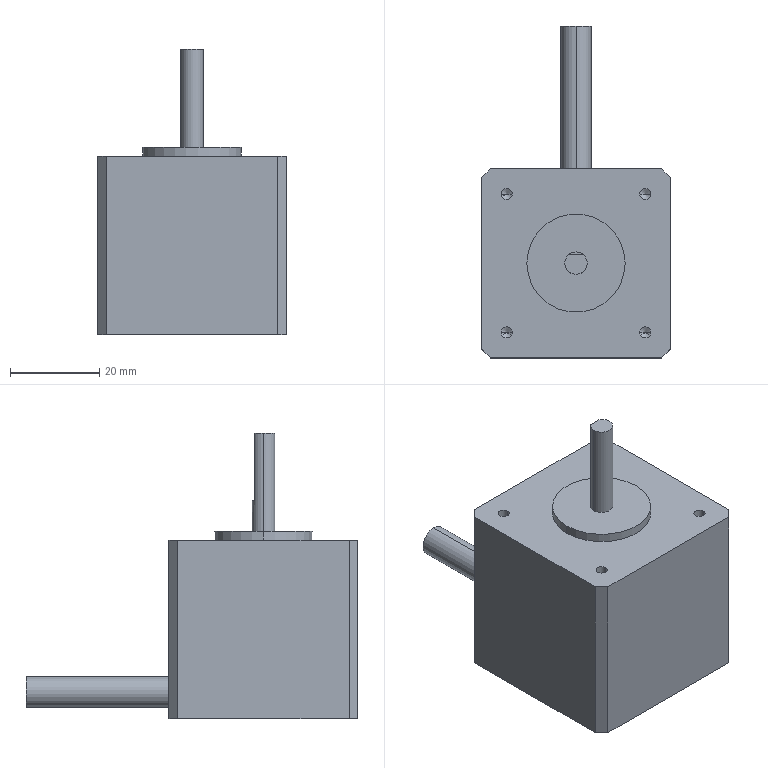Part | NX | features BREP 1 | 1 solid | 37 faces | box 42.3 x 74.3 x 64 mm | volume 73352 mm3 | plane 15 | cylinder 14 | cone 8 | commonest cylinder face diameters 2.5 x8 5 x2 6.776 x2 22 x2
STEP:
#1=CARTESIAN_POINT('',(0.,53.15,2.645));
#2=VERTEX_POINT('',#1);
#3=CARTESIAN_POINT('',(0.,53.15,9.422));
#4=VERTEX_POINT('',#3);
#5=CARTESIAN_POINT('',(0.,53.15,6.033));
#6=DIRECTION('',(0.,1.,0.));
#7=DIRECTION('',(0.,0.,1.));
#8=AXIS2_PLACEMENT_3D('',#5,#6,#7);
#9=CIRCLE('',#8,3.388);
#10=EDGE_CURVE('',#2,#4,#9,.T.);
#11=ORIENTED_EDGE('',*,*,#10,.T.);
#12=CARTESIAN_POINT('',(0.,53.15,6.033));
#13=DIRECTION('',(0.,1.,0.));
#14=DIRECTION('',(0.,0.,1.));
#15=AXIS2_PLACEMENT_3D('',#12,#13,#14);
#16=CIRCLE('',#15,3.388);
#17=EDGE_CURVE('',#4,#2,#16,.T.);
#18=ORIENTED_EDGE('',*,*,#17,.T.);
#19=EDGE_LOOP('',(#11,#18));
#20=FACE_BOUND('',#19,.T.);
#21=CARTESIAN_POINT('',(0.,53.15,6.033));
#22=DIRECTION('',(0.,1.,0.));
#23=DIRECTION('',(0.,0.,1.));
#24=AXIS2_PLACEMENT_3D('',#21,#22,#23);
#25=PLANE('',#24);
#26=ADVANCED_FACE('',(#20),#25,.T.);
#27=CARTESIAN_POINT('',(0.,21.15,9.422));
#28=VERTEX_POINT('',#27);
#29=CARTESIAN_POINT('',(0.,53.15,9.422));
#30=DIRECTION('',(0.,-1.,0.));
#31=VECTOR('',#30,1000.);
#32=LINE('',#29,#31);
#33=EDGE_CURVE('',#4,#28,#32,.T.);
#34=ORIENTED_EDGE('',*,*,#33,.F.);
#35=ORIENTED_EDGE('',*,*,#10,.F.);
#36=CARTESIAN_POINT('',(0.,21.15,2.645));
#37=VERTEX_POINT('',#36);
#38=CARTESIAN_POINT('',(0.,53.15,2.645));
#39=DIRECTION('',(0.,-1.,0.));
#40=VECTOR('',#39,1000.);
#41=LINE('',#38,#40);
#42=EDGE_CURVE('',#2,#37,#41,.T.);
#43=ORIENTED_EDGE('',*,*,#42,.T.);
#44=CARTESIAN_POINT('',(0.,21.15,6.033));
#45=DIRECTION('',(0.,1.,0.));
#46=DIRECTION('',(0.,0.,-1.));
#47=AXIS2_PLACEMENT_3D('',#44,#45,#46);
#48=CIRCLE('',#47,3.388);
#49=EDGE_CURVE('',#37,#28,#48,.T.);
#50=ORIENTED_EDGE('',*,*,#49,.T.);
#51=EDGE_LOOP('',(#34,#35,#43,#50));
#52=FACE_BOUND('',#51,.T.);
#53=CARTESIAN_POINT('',(0.,53.15,6.033));
#54=DIRECTION('',(0.,-1.,0.));
#55=DIRECTION('',(0.,0.,-1.));
#56=AXIS2_PLACEMENT_3D('',#53,#54,#55);
#57=CYLINDRICAL_SURFACE('',#56,3.388);
#58=ADVANCED_FACE('',(#52),#57,.T.);
#59=CARTESIAN_POINT('',(-19.15,21.15,40.));
#60=VERTEX_POINT('',#59);
#61=CARTESIAN_POINT('',(-21.15,19.15,40.));
#62=VERTEX_POINT('',#61);
#63=CARTESIAN_POINT('',(-21.15,19.15,40.));
#64=DIRECTION('',(-0.7071,-0.7071,0.));
#65=VECTOR('',#64,1000.);
#66=LINE('',#63,#65);
#67=EDGE_CURVE('',#60,#62,#66,.T.);
#68=ORIENTED_EDGE('',*,*,#67,.F.);
#69=CARTESIAN_POINT('',(-19.15,21.15,0.));
#70=VERTEX_POINT('',#69);
#71=CARTESIAN_POINT('',(-19.15,21.15,40.));
#72=DIRECTION('',(0.,0.,1.));
#73=VECTOR('',#72,1000.);
#74=LINE('',#71,#73);
#75=EDGE_CURVE('',#70,#60,#74,.T.);
#76=ORIENTED_EDGE('',*,*,#75,.F.);
#77=CARTESIAN_POINT('',(-21.15,19.15,0.));
#78=VERTEX_POINT('',#77);
#79=CARTESIAN_POINT('',(-20.15,20.15,0.));
#80=DIRECTION('',(0.7071,0.7071,0.));
#81=VECTOR('',#80,1000.);
#82=LINE('',#79,#81);
#83=EDGE_CURVE('',#78,#70,#82,.T.);
#84=ORIENTED_EDGE('',*,*,#83,.F.);
#85=CARTESIAN_POINT('',(-21.15,19.15,40.));
#86=DIRECTION('',(0.,0.,-1.));
#87=VECTOR('',#86,1000.);
#88=LINE('',#85,#87);
#89=EDGE_CURVE('',#62,#78,#88,.T.);
#90=ORIENTED_EDGE('',*,*,#89,.F.);
#91=EDGE_LOOP('',(#68,#76,#84,#90));
#92=FACE_BOUND('',#91,.T.);
#93=CARTESIAN_POINT('',(-21.15,19.15,40.));
#94=DIRECTION('',(0.7071,-0.7071,0.));
#95=DIRECTION('',(0.,0.,-1.));
#96=AXIS2_PLACEMENT_3D('',#93,#94,#95);
#97=PLANE('',#96);
#98=ADVANCED_FACE('',(#92),#97,.F.);
#99=CARTESIAN_POINT('',(21.15,19.15,40.));
#100=VERTEX_POINT('',#99);
#101=CARTESIAN_POINT('',(19.15,21.15,40.));
#102=VERTEX_POINT('',#101);
#103=CARTESIAN_POINT('',(19.15,21.15,40.));
#104=DIRECTION('',(-0.7071,0.7071,0.));
#105=VECTOR('',#104,1000.);
#106=LINE('',#103,#105);
#107=EDGE_CURVE('',#100,#102,#106,.T.);
#108=ORIENTED_EDGE('',*,*,#107,.F.);
#109=CARTESIAN_POINT('',(21.15,19.15,0.));
#110=VERTEX_POINT('',#109);
#111=CARTESIAN_POINT('',(21.15,19.15,40.));
#112=DIRECTION('',(0.,0.,1.));
#113=VECTOR('',#112,1000.);
#114=LINE('',#111,#113);
#115=EDGE_CURVE('',#110,#100,#114,.T.);
#116=ORIENTED_EDGE('',*,*,#115,.F.);
#117=CARTESIAN_POINT('',(19.15,21.15,0.));
#118=VERTEX_POINT('',#117);
#119=CARTESIAN_POINT('',(20.15,20.15,0.));
#120=DIRECTION('',(0.7071,-0.7071,0.));
#121=VECTOR('',#120,1000.);
#122=LINE('',#119,#121);
#123=EDGE_CURVE('',#118,#110,#122,.T.);
#124=ORIENTED_EDGE('',*,*,#123,.F.);
#125=CARTESIAN_POINT('',(19.15,21.15,40.));
#126=DIRECTION('',(0.,0.,-1.));
#127=VECTOR('',#126,1000.);
#128=LINE('',#125,#127);
#129=EDGE_CURVE('',#102,#118,#128,.T.);
#130=ORIENTED_EDGE('',*,*,#129,.F.);
#131=EDGE_LOOP('',(#108,#116,#124,#130));
#132=FACE_BOUND('',#131,.T.);
#133=CARTESIAN_POINT('',(19.15,21.15,40.));
#134=DIRECTION('',(-0.7071,-0.7071,0.));
#135=DIRECTION('',(0.,0.,-1.));
#136=AXIS2_PLACEMENT_3D('',#133,#134,#135);
#137=PLANE('',#136);
#138=ADVANCED_FACE('',(#132),#137,.F.);
#139=CARTESIAN_POINT('',(-21.15,-19.15,40.));
#140=VERTEX_POINT('',#139);
#141=CARTESIAN_POINT('',(-19.15,-21.15,40.));
#142=VERTEX_POINT('',#141);
#143=CARTESIAN_POINT('',(-19.15,-21.15,40.));
#144=DIRECTION('',(0.7071,-0.7071,0.));
#145=VECTOR('',#144,1000.);
#146=LINE('',#143,#145);
#147=EDGE_CURVE('',#140,#142,#146,.T.);
#148=ORIENTED_EDGE('',*,*,#147,.F.);
#149=CARTESIAN_POINT('',(-21.15,-19.15,0.));
#150=VERTEX_POINT('',#149);
#151=CARTESIAN_POINT('',(-21.15,-19.15,40.));
#152=DIRECTION('',(0.,0.,1.));
#153=VECTOR('',#152,1000.);
#154=LINE('',#151,#153);
#155=EDGE_CURVE('',#150,#140,#154,.T.);
#156=ORIENTED_EDGE('',*,*,#155,.F.);
#157=CARTESIAN_POINT('',(-19.15,-21.15,0.));
#158=VERTEX_POINT('',#157);
#159=CARTESIAN_POINT('',(-20.15,-20.15,0.));
#160=DIRECTION('',(-0.7071,0.7071,0.));
#161=VECTOR('',#160,1000.);
#162=LINE('',#159,#161);
#163=EDGE_CURVE('',#158,#150,#162,.T.);
#164=ORIENTED_EDGE('',*,*,#163,.F.);
#165=CARTESIAN_POINT('',(-19.15,-21.15,40.));
#166=DIRECTION('',(0.,0.,-1.));
#167=VECTOR('',#166,1000.);
#168=LINE('',#165,#167);
#169=EDGE_CURVE('',#142,#158,#168,.T.);
#170=ORIENTED_EDGE('',*,*,#169,.F.);
#171=EDGE_LOOP('',(#148,#156,#164,#170));
#172=FACE_BOUND('',#171,.T.);
#173=CARTESIAN_POINT('',(-19.15,-21.15,40.));
#174=DIRECTION('',(0.7071,0.7071,0.));
#175=DIRECTION('',(0.,0.,-1.));
#176=AXIS2_PLACEMENT_3D('',#173,#174,#175);
#177=PLANE('',#176);
#178=ADVANCED_FACE('',(#172),#177,.F.);
#179=CARTESIAN_POINT('',(19.15,-21.15,40.));
#180=VERTEX_POINT('',#179);
#181=CARTESIAN_POINT('',(21.15,-19.15,40.));
#182=VERTEX_POINT('',#181);
#183=CARTESIAN_POINT('',(21.15,-19.15,40.));
#184=DIRECTION('',(0.7071,0.7071,0.));
#185=VECTOR('',#184,1000.);
#186=LINE('',#183,#185);
#187=EDGE_CURVE('',#180,#182,#186,.T.);
#188=ORIENTED_EDGE('',*,*,#187,.F.);
#189=CARTESIAN_POINT('',(19.15,-21.15,0.));
#190=VERTEX_POINT('',#189);
#191=CARTESIAN_POINT('',(19.15,-21.15,40.));
#192=DIRECTION('',(0.,0.,1.));
#193=VECTOR('',#192,1000.);
#194=LINE('',#191,#193);
#195=EDGE_CURVE('',#190,#180,#194,.T.);
#196=ORIENTED_EDGE('',*,*,#195,.F.);
#197=CARTESIAN_POINT('',(21.15,-19.15,0.));
#198=VERTEX_POINT('',#197);
#199=CARTESIAN_POINT('',(20.15,-20.15,0.));
#200=DIRECTION('',(-0.7071,-0.7071,0.));
#201=VECTOR('',#200,1000.);
#202=LINE('',#199,#201);
#203=EDGE_CURVE('',#198,#190,#202,.T.);
#204=ORIENTED_EDGE('',*,*,#203,.F.);
#205=CARTESIAN_POINT('',(21.15,-19.15,40.));
#206=DIRECTION('',(0.,0.,-1.));
#207=VECTOR('',#206,1000.);
#208=LINE('',#205,#207);
#209=EDGE_CURVE('',#182,#198,#208,.T.);
#210=ORIENTED_EDGE('',*,*,#209,.F.);
#211=EDGE_LOOP('',(#188,#196,#204,#210));
#212=FACE_BOUND('',#211,.T.);
#213=CARTESIAN_POINT('',(21.15,-19.15,40.));
#214=DIRECTION('',(-0.7071,0.7071,0.));
#215=DIRECTION('',(0.,0.,-1.));
#216=AXIS2_PLACEMENT_3D('',#213,#214,#215);
#217=PLANE('',#216);
#218=ADVANCED_FACE('',(#212),#217,.F.);
#219=CARTESIAN_POINT('',(-16.75,15.5,40.));
#220=VERTEX_POINT('',#219);
#221=CARTESIAN_POINT('',(-16.75,15.5,28.5));
#222=VERTEX_POINT('',#221);
#223=CARTESIAN_POINT('',(-16.75,15.5,40.));
#224=DIRECTION('',(0.,0.,1.));
#225=VECTOR('',#224,1000.);
#226=LINE('',#223,#225);
#227=EDGE_CURVE('',#220,#222,#226,.F.);
#228=ORIENTED_EDGE('',*,*,#227,.T.);
#229=CARTESIAN_POINT('',(-14.25,15.5,28.5));
#230=VERTEX_POINT('',#229);
#231=CARTESIAN_POINT('',(-15.5,15.5,28.5));
#232=DIRECTION('',(0.,0.,1.));
#233=DIRECTION('',(1.,0.,0.));
#234=AXIS2_PLACEMENT_3D('',#231,#232,#233);
#235=CIRCLE('',#234,1.25);
#236=EDGE_CURVE('',#230,#222,#235,.T.);
#237=ORIENTED_EDGE('',*,*,#236,.F.);
#238=CARTESIAN_POINT('',(-14.25,15.5,40.));
#239=VERTEX_POINT('',#238);
#240=CARTESIAN_POINT('',(-14.25,15.5,40.));
#241=DIRECTION('',(0.,0.,1.));
#242=VECTOR('',#241,1000.);
#243=LINE('',#240,#242);
#244=EDGE_CURVE('',#239,#230,#243,.F.);
#245=ORIENTED_EDGE('',*,*,#244,.F.);
#246=CARTESIAN_POINT('',(-15.5,15.5,40.));
#247=DIRECTION('',(0.,0.,1.));
#248=DIRECTION('',(1.,0.,0.));
#249=AXIS2_PLACEMENT_3D('',#246,#247,#248);
#250=CIRCLE('',#249,1.25);
#251=EDGE_CURVE('',#239,#220,#250,.T.);
#252=ORIENTED_EDGE('',*,*,#251,.T.);
#253=EDGE_LOOP('',(#228,#237,#245,#252));
#254=FACE_BOUND('',#253,.T.);
#255=CARTESIAN_POINT('',(-15.5,15.5,40.));
#256=DIRECTION('',(0.,0.,1.));
#257=DIRECTION('',(1.,0.,0.));
#258=AXIS2_PLACEMENT_3D('',#255,#256,#257);
#259=CYLINDRICAL_SURFACE('',#258,1.25);
#260=ADVANCED_FACE('',(#254),#259,.F.);
#261=CARTESIAN_POINT('',(-15.5,15.5,27.749));
#262=VERTEX_POINT('',#261);
#263=CARTESIAN_POINT('',(-16.75,15.5,28.5));
#264=DIRECTION('',(-0.8572,0.,0.515));
#265=VECTOR('',#264,1000.);
#266=LINE('',#263,#265);
#267=EDGE_CURVE('',#262,#222,#266,.T.);
#268=ORIENTED_EDGE('',*,*,#267,.F.);
#269=CARTESIAN_POINT('',(-14.25,15.5,28.5));
#270=DIRECTION('',(0.8572,0.,0.515));
#271=VECTOR('',#270,1000.);
#272=LINE('',#269,#271);
#273=EDGE_CURVE('',#262,#230,#272,.T.);
#274=ORIENTED_EDGE('',*,*,#273,.T.);
#275=ORIENTED_EDGE('',*,*,#236,.T.);
#276=EDGE_LOOP('',(#268,#274,#275));
#277=FACE_BOUND('',#276,.T.);
#278=CARTESIAN_POINT('',(-15.5,15.5,28.5));
#279=DIRECTION('',(0.,0.,1.));
#280=DIRECTION('',(1.,0.,0.));
#281=AXIS2_PLACEMENT_3D('',#278,#279,#280);
#282=CONICAL_SURFACE('',#281,1.25,1.03);
#283=ADVANCED_FACE('',(#277),#282,.F.);
#284=CARTESIAN_POINT('',(14.25,15.5,40.));
#285=VERTEX_POINT('',#284);
#286=CARTESIAN_POINT('',(14.25,15.5,28.5));
#287=VERTEX_POINT('',#286);
#288=CARTESIAN_POINT('',(14.25,15.5,40.));
#289=DIRECTION('',(0.,0.,1.));
#290=VECTOR('',#289,1000.);
#291=LINE('',#288,#290);
#292=EDGE_CURVE('',#285,#287,#291,.F.);
#293=ORIENTED_EDGE('',*,*,#292,.T.);
#294=CARTESIAN_POINT('',(16.75,15.5,28.5));
#295=VERTEX_POINT('',#294);
#296=CARTESIAN_POINT('',(15.5,15.5,28.5));
#297=DIRECTION('',(0.,0.,1.));
#298=DIRECTION('',(1.,0.,0.));
#299=AXIS2_PLACEMENT_3D('',#296,#297,#298);
#300=CIRCLE('',#299,1.25);
#301=EDGE_CURVE('',#295,#287,#300,.T.);
#302=ORIENTED_EDGE('',*,*,#301,.F.);
#303=CARTESIAN_POINT('',(16.75,15.5,40.));
#304=VERTEX_POINT('',#303);
#305=CARTESIAN_POINT('',(16.75,15.5,40.));
#306=DIRECTION('',(0.,0.,1.));
#307=VECTOR('',#306,1000.);
#308=LINE('',#305,#307);
#309=EDGE_CURVE('',#304,#295,#308,.F.);
#310=ORIENTED_EDGE('',*,*,#309,.F.);
#311=CARTESIAN_POINT('',(15.5,15.5,40.));
#312=DIRECTION('',(0.,0.,1.));
#313=DIRECTION('',(1.,0.,0.));
#314=AXIS2_PLACEMENT_3D('',#311,#312,#313);
#315=CIRCLE('',#314,1.25);
#316=EDGE_CURVE('',#304,#285,#315,.T.);
#317=ORIENTED_EDGE('',*,*,#316,.T.);
#318=EDGE_LOOP('',(#293,#302,#310,#317));
#319=FACE_BOUND('',#318,.T.);
#320=CARTESIAN_POINT('',(15.5,15.5,40.));
#321=DIRECTION('',(0.,0.,1.));
#322=DIRECTION('',(1.,0.,0.));
#323=AXIS2_PLACEMENT_3D('',#320,#321,#322);
#324=CYLINDRICAL_SURFACE('',#323,1.25);
#325=ADVANCED_FACE('',(#319),#324,.F.);
#326=CARTESIAN_POINT('',(15.5,15.5,27.749));
#327=VERTEX_POINT('',#326);
#328=CARTESIAN_POINT('',(14.25,15.5,28.5));
#329=DIRECTION('',(-0.8572,0.,0.515));
#330=VECTOR('',#329,1000.);
#331=LINE('',#328,#330);
#332=EDGE_CURVE('',#327,#287,#331,.T.);
#333=ORIENTED_EDGE('',*,*,#332,.F.);
#334=CARTESIAN_POINT('',(16.75,15.5,28.5));
#335=DIRECTION('',(0.8572,0.,0.515));
#336=VECTOR('',#335,1000.);
#337=LINE('',#334,#336);
#338=EDGE_CURVE('',#327,#295,#337,.T.);
#339=ORIENTED_EDGE('',*,*,#338,.T.);
#340=ORIENTED_EDGE('',*,*,#301,.T.);
#341=EDGE_LOOP('',(#333,#339,#340));
#342=FACE_BOUND('',#341,.T.);
#343=CARTESIAN_POINT('',(15.5,15.5,28.5));
#344=DIRECTION('',(0.,0.,1.));
#345=DIRECTION('',(1.,0.,0.));
#346=AXIS2_PLACEMENT_3D('',#343,#344,#345);
#347=CONICAL_SURFACE('',#346,1.25,1.03);
#348=ADVANCED_FACE('',(#342),#347,.F.);
#349=CARTESIAN_POINT('',(14.25,-15.5,40.));
#350=VERTEX_POINT('',#349);
#351=CARTESIAN_POINT('',(14.25,-15.5,28.5));
#352=VERTEX_POINT('',#351);
#353=CARTESIAN_POINT('',(14.25,-15.5,40.));
#354=DIRECTION('',(0.,0.,1.));
#355=VECTOR('',#354,1000.);
#356=LINE('',#353,#355);
#357=EDGE_CURVE('',#350,#352,#356,.F.);
#358=ORIENTED_EDGE('',*,*,#357,.T.);
#359=CARTESIAN_POINT('',(16.75,-15.5,28.5));
#360=VERTEX_POINT('',#359);
#361=CARTESIAN_POINT('',(15.5,-15.5,28.5));
#362=DIRECTION('',(0.,0.,1.));
#363=DIRECTION('',(1.,0.,0.));
#364=AXIS2_PLACEMENT_3D('',#361,#362,#363);
#365=CIRCLE('',#364,1.25);
#366=EDGE_CURVE('',#360,#352,#365,.T.);
#367=ORIENTED_EDGE('',*,*,#366,.F.);
#368=CARTESIAN_POINT('',(16.75,-15.5,40.));
#369=VERTEX_POINT('',#368);
#370=CARTESIAN_POINT('',(16.75,-15.5,40.));
#371=DIRECTION('',(0.,0.,1.));
#372=VECTOR('',#371,1000.);
#373=LINE('',#370,#372);
#374=EDGE_CURVE('',#369,#360,#373,.F.);
#375=ORIENTED_EDGE('',*,*,#374,.F.);
#376=CARTESIAN_POINT('',(15.5,-15.5,40.));
#377=DIRECTION('',(0.,0.,1.));
#378=DIRECTION('',(1.,0.,0.));
#379=AXIS2_PLACEMENT_3D('',#376,#377,#378);
#380=CIRCLE('',#379,1.25);
#381=EDGE_CURVE('',#369,#350,#380,.T.);
#382=ORIENTED_EDGE('',*,*,#381,.T.);
#383=EDGE_LOOP('',(#358,#367,#375,#382));
#384=FACE_BOUND('',#383,.T.);
#385=CARTESIAN_POINT('',(15.5,-15.5,40.));
#386=DIRECTION('',(0.,0.,1.));
#387=DIRECTION('',(1.,0.,0.));
#388=AXIS2_PLACEMENT_3D('',#385,#386,#387);
#389=CYLINDRICAL_SURFACE('',#388,1.25);
#390=ADVANCED_FACE('',(#384),#389,.F.);
#391=CARTESIAN_POINT('',(15.5,-15.5,27.749));
#392=VERTEX_POINT('',#391);
#393=CARTESIAN_POINT('',(14.25,-15.5,28.5));
#394=DIRECTION('',(-0.8572,0.,0.515));
#395=VECTOR('',#394,1000.);
#396=LINE('',#393,#395);
#397=EDGE_CURVE('',#392,#352,#396,.T.);
#398=ORIENTED_EDGE('',*,*,#397,.F.);
#399=CARTESIAN_POINT('',(16.75,-15.5,28.5));
#400=DIRECTION('',(0.8572,0.,0.515));
#401=VECTOR('',#400,1000.);
#402=LINE('',#399,#401);
#403=EDGE_CURVE('',#392,#360,#402,.T.);
#404=ORIENTED_EDGE('',*,*,#403,.T.);
#405=ORIENTED_EDGE('',*,*,#366,.T.);
#406=EDGE_LOOP('',(#398,#404,#405));
#407=FACE_BOUND('',#406,.T.);
#408=CARTESIAN_POINT('',(15.5,-15.5,28.5));
#409=DIRECTION('',(0.,0.,1.));
#410=DIRECTION('',(1.,0.,0.));
#411=AXIS2_PLACEMENT_3D('',#408,#409,#410);
#412=CONICAL_SURFACE('',#411,1.25,1.03);
#413=ADVANCED_FACE('',(#407),#412,.F.);
#414=CARTESIAN_POINT('',(-16.75,-15.5,40.));
#415=VERTEX_POINT('',#414);
#416=CARTESIAN_POINT('',(-16.75,-15.5,28.5));
#417=VERTEX_POINT('',#416);
#418=CARTESIAN_POINT('',(-16.75,-15.5,40.));
#419=DIRECTION('',(0.,0.,1.));
#420=VECTOR('',#419,1000.);
#421=LINE('',#418,#420);
#422=EDGE_CURVE('',#415,#417,#421,.F.);
#423=ORIENTED_EDGE('',*,*,#422,.T.);
#424=CARTESIAN_POINT('',(-14.25,-15.5,28.5));
#425=VERTEX_POINT('',#424);
#426=CARTESIAN_POINT('',(-15.5,-15.5,28.5));
#427=DIRECTION('',(0.,0.,1.));
#428=DIRECTION('',(1.,0.,0.));
#429=AXIS2_PLACEMENT_3D('',#426,#427,#428);
#430=CIRCLE('',#429,1.25);
#431=EDGE_CURVE('',#425,#417,#430,.T.);
#432=ORIENTED_EDGE('',*,*,#431,.F.);
#433=CARTESIAN_POINT('',(-14.25,-15.5,40.));
#434=VERTEX_POINT('',#433);
#435=CARTESIAN_POINT('',(-14.25,-15.5,40.));
#436=DIRECTION('',(0.,0.,1.));
#437=VECTOR('',#436,1000.);
#438=LINE('',#435,#437);
#439=EDGE_CURVE('',#434,#425,#438,.F.);
#440=ORIENTED_EDGE('',*,*,#439,.F.);
#441=CARTESIAN_POINT('',(-15.5,-15.5,40.));
#442=DIRECTION('',(0.,0.,1.));
#443=DIRECTION('',(1.,0.,0.));
#444=AXIS2_PLACEMENT_3D('',#441,#442,#443);
#445=CIRCLE('',#444,1.25);
#446=EDGE_CURVE('',#434,#415,#445,.T.);
#447=ORIENTED_EDGE('',*,*,#446,.T.);
#448=EDGE_LOOP('',(#423,#432,#440,#447));
#449=FACE_BOUND('',#448,.T.);
#450=CARTESIAN_POINT('',(-15.5,-15.5,40.));
#451=DIRECTION('',(0.,0.,1.));
#452=DIRECTION('',(1.,0.,0.));
#453=AXIS2_PLACEMENT_3D('',#450,#451,#452);
#454=CYLINDRICAL_SURFACE('',#453,1.25);
#455=ADVANCED_FACE('',(#449),#454,.F.);
#456=CARTESIAN_POINT('',(-15.5,-15.5,27.749));
#457=VERTEX_POINT('',#456);
#458=CARTESIAN_POINT('',(-16.75,-15.5,28.5));
#459=DIRECTION('',(-0.8572,0.,0.515));
#460=VECTOR('',#459,1000.);
#461=LINE('',#458,#460);
#462=EDGE_CURVE('',#457,#417,#461,.T.);
#463=ORIENTED_EDGE('',*,*,#462,.F.);
#464=CARTESIAN_POINT('',(-14.25,-15.5,28.5));
#465=DIRECTION('',(0.8572,0.,0.515));
#466=VECTOR('',#465,1000.);
#467=LINE('',#464,#466);
#468=EDGE_CURVE('',#457,#425,#467,.T.);
#469=ORIENTED_EDGE('',*,*,#468,.T.);
#470=ORIENTED_EDGE('',*,*,#431,.T.);
#471=EDGE_LOOP('',(#463,#469,#470));
#472=FACE_BOUND('',#471,.T.);
#473=CARTESIAN_POINT('',(-15.5,-15.5,28.5));
#474=DIRECTION('',(0.,0.,1.));
#475=DIRECTION('',(1.,0.,0.));
#476=AXIS2_PLACEMENT_3D('',#473,#474,#475);
#477=CONICAL_SURFACE('',#476,1.25,1.03);
#478=ADVANCED_FACE('',(#472),#477,.F.);
#479=CARTESIAN_POINT('',(-1.5,2.,64.));
#480=VERTEX_POINT('',#479);
#481=CARTESIAN_POINT('',(1.5,2.,64.));
#482=VERTEX_POINT('',#481);
#483=CARTESIAN_POINT('',(-1.5,2.,64.));
#484=DIRECTION('',(1.,0.,0.));
#485=VECTOR('',#484,1000.);
#486=LINE('',#483,#485);
#487=EDGE_CURVE('',#480,#482,#486,.T.);
#488=ORIENTED_EDGE('',*,*,#487,.T.);
#489=CARTESIAN_POINT('',(1.5,2.,49.));
#490=VERTEX_POINT('',#489);
#491=CARTESIAN_POINT('',(1.5,2.,49.));
#492=DIRECTION('',(0.,0.,1.));
#493=VECTOR('',#492,1000.);
#494=LINE('',#491,#493);
#495=EDGE_CURVE('',#482,#490,#494,.F.);
#496=ORIENTED_EDGE('',*,*,#495,.T.);
#497=CARTESIAN_POINT('',(-1.5,2.,49.));
#498=VERTEX_POINT('',#497);
#499=CARTESIAN_POINT('',(-1.5,2.,49.));
#500=DIRECTION('',(1.,0.,0.));
#501=VECTOR('',#500,1000.);
#502=LINE('',#499,#501);
#503=EDGE_CURVE('',#498,#490,#502,.T.);
#504=ORIENTED_EDGE('',*,*,#503,.F.);
#505=CARTESIAN_POINT('',(-1.5,2.,49.));
#506=DIRECTION('',(0.,0.,1.));
#507=VECTOR('',#506,1000.);
#508=LINE('',#505,#507);
#509=EDGE_CURVE('',#480,#498,#508,.F.);
#510=ORIENTED_EDGE('',*,*,#509,.F.);
#511=EDGE_LOOP('',(#488,#496,#504,#510));
#512=FACE_BOUND('',#511,.T.);
#513=CARTESIAN_POINT('',(-1.5,2.,49.));
#514=DIRECTION('',(0.,-1.,0.));
#515=DIRECTION('',(0.,0.,-1.));
#516=AXIS2_PLACEMENT_3D('',#513,#514,#515);
#517=PLANE('',#516);
#518=ADVANCED_FACE('',(#512),#517,.F.);
#519=ORIENTED_EDGE('',*,*,#503,.T.);
#520=CARTESIAN_POINT('',(0.,0.,49.));
#521=DIRECTION('',(0.,0.,-1.));
#522=DIRECTION('',(-1.,0.,0.));
#523=AXIS2_PLACEMENT_3D('',#520,#521,#522);
#524=CIRCLE('',#523,2.5);
#525=EDGE_CURVE('',#498,#490,#524,.T.);
#526=ORIENTED_EDGE('',*,*,#525,.F.);
#527=EDGE_LOOP('',(#519,#526));
#528=FACE_BOUND('',#527,.T.);
#529=CARTESIAN_POINT('',(0.,0.,49.));
#530=DIRECTION('',(0.,0.,-1.));
#531=DIRECTION('',(-1.,0.,0.));
#532=AXIS2_PLACEMENT_3D('',#529,#530,#531);
#533=PLANE('',#532);
#534=ADVANCED_FACE('',(#528),#533,.F.);
#535=ORIENTED_EDGE('',*,*,#487,.F.);
#536=CARTESIAN_POINT('',(-2.5,0.,64.));
#537=VERTEX_POINT('',#536);
#538=CARTESIAN_POINT('',(0.,0.,64.));
#539=DIRECTION('',(0.,0.,1.));
#540=DIRECTION('',(1.,0.,0.));
#541=AXIS2_PLACEMENT_3D('',#538,#539,#540);
#542=CIRCLE('',#541,2.5);
#543=EDGE_CURVE('',#480,#537,#542,.T.);
#544=ORIENTED_EDGE('',*,*,#543,.T.);
#545=CARTESIAN_POINT('',(2.5,0.,64.));
#546=VERTEX_POINT('',#545);
#547=CARTESIAN_POINT('',(0.,0.,64.));
#548=DIRECTION('',(0.,0.,1.));
#549=DIRECTION('',(1.,0.,0.));
#550=AXIS2_PLACEMENT_3D('',#547,#548,#549);
#551=CIRCLE('',#550,2.5);
#552=EDGE_CURVE('',#537,#546,#551,.T.);
#553=ORIENTED_EDGE('',*,*,#552,.T.);
#554=CARTESIAN_POINT('',(0.,0.,64.));
#555=DIRECTION('',(0.,0.,1.));
#556=DIRECTION('',(1.,0.,0.));
#557=AXIS2_PLACEMENT_3D('',#554,#555,#556);
#558=CIRCLE('',#557,2.5);
#559=EDGE_CURVE('',#546,#482,#558,.T.);
#560=ORIENTED_EDGE('',*,*,#559,.T.);
#561=EDGE_LOOP('',(#535,#544,#553,#560));
#562=FACE_BOUND('',#561,.T.);
#563=CARTESIAN_POINT('',(0.,0.,64.));
#564=DIRECTION('',(0.,0.,1.));
#565=DIRECTION('',(1.,0.,0.));
#566=AXIS2_PLACEMENT_3D('',#563,#564,#565);
#567=PLANE('',#566);
#568=ADVANCED_FACE('',(#562),#567,.T.);
#569=CARTESIAN_POINT('',(2.5,0.,42.));
#570=VERTEX_POINT('',#569);
#571=CARTESIAN_POINT('',(2.5,0.,64.));
#572=DIRECTION('',(0.,0.,-1.));
#573=VECTOR('',#572,1000.);
#574=LINE('',#571,#573);
#575=EDGE_CURVE('',#546,#570,#574,.T.);
#576=ORIENTED_EDGE('',*,*,#575,.F.);
#577=ORIENTED_EDGE('',*,*,#552,.F.);
#578=CARTESIAN_POINT('',(-2.5,0.,42.));
#579=VERTEX_POINT('',#578);
#580=CARTESIAN_POINT('',(-2.5,0.,64.));
#581=DIRECTION('',(0.,0.,-1.));
#582=VECTOR('',#581,1000.);
#583=LINE('',#580,#582);
#584=EDGE_CURVE('',#537,#579,#583,.T.);
#585=ORIENTED_EDGE('',*,*,#584,.T.);
#586=CARTESIAN_POINT('',(0.,0.,42.));
#587=DIRECTION('',(0.,0.,-1.));
#588=DIRECTION('',(1.,0.,0.));
#589=AXIS2_PLACEMENT_3D('',#586,#587,#588);
#590=CIRCLE('',#589,2.5);
#591=EDGE_CURVE('',#570,#579,#590,.T.);
#592=ORIENTED_EDGE('',*,*,#591,.F.);
#593=EDGE_LOOP('',(#576,#577,#585,#592));
#594=FACE_BOUND('',#593,.T.);
#595=CARTESIAN_POINT('',(0.,0.,64.));
#596=DIRECTION('',(0.,0.,-1.));
#597=DIRECTION('',(-1.,0.,0.));
#598=AXIS2_PLACEMENT_3D('',#595,#596,#597);
#599=CYLINDRICAL_SURFACE('',#598,2.5);
#600=ADVANCED_FACE('',(#594),#599,.T.);
#601=CARTESIAN_POINT('',(-11.,0.,42.));
#602=VERTEX_POINT('',#601);
#603=CARTESIAN_POINT('',(11.,0.,42.));
#604=VERTEX_POINT('',#603);
#605=CARTESIAN_POINT('',(0.,0.,42.));
#606=DIRECTION('',(0.,0.,1.));
#607=DIRECTION('',(1.,0.,0.));
#608=AXIS2_PLACEMENT_3D('',#605,#606,#607);
#609=CIRCLE('',#608,11.);
#610=EDGE_CURVE('',#602,#604,#609,.T.);
#611=ORIENTED_EDGE('',*,*,#610,.T.);
#612=CARTESIAN_POINT('',(0.,0.,42.));
#613=DIRECTION('',(0.,0.,1.));
#614=DIRECTION('',(1.,0.,0.));
#615=AXIS2_PLACEMENT_3D('',#612,#613,#614);
#616=CIRCLE('',#615,11.);
#617=EDGE_CURVE('',#604,#602,#616,.T.);
#618=ORIENTED_EDGE('',*,*,#617,.T.);
#619=EDGE_LOOP('',(#611,#618));
#620=FACE_BOUND('',#619,.T.);
#621=CARTESIAN_POINT('',(0.,0.,42.));
#622=DIRECTION('',(0.,0.,-1.));
#623=DIRECTION('',(1.,0.,0.));
#624=AXIS2_PLACEMENT_3D('',#621,#622,#623);
#625=CIRCLE('',#624,2.5);
#626=EDGE_CURVE('',#579,#570,#625,.T.);
#627=ORIENTED_EDGE('',*,*,#626,.T.);
#628=ORIENTED_EDGE('',*,*,#591,.T.);
#629=EDGE_LOOP('',(#627,#628));
#630=FACE_BOUND('',#629,.T.);
#631=CARTESIAN_POINT('',(0.,0.,42.));
#632=DIRECTION('',(0.,0.,1.));
#633=DIRECTION('',(1.,0.,0.));
#634=AXIS2_PLACEMENT_3D('',#631,#632,#633);
#635=PLANE('',#634);
#636=ADVANCED_FACE('',(#620,#630),#635,.T.);
#637=CARTESIAN_POINT('',(11.,0.,40.));
#638=VERTEX_POINT('',#637);
#639=CARTESIAN_POINT('',(11.,0.,42.));
#640=DIRECTION('',(0.,0.,-1.));
#641=VECTOR('',#640,1000.);
#642=LINE('',#639,#641);
#643=EDGE_CURVE('',#604,#638,#642,.T.);
#644=ORIENTED_EDGE('',*,*,#643,.F.);
#645=ORIENTED_EDGE('',*,*,#610,.F.);
#646=CARTESIAN_POINT('',(-11.,0.,40.));
#647=VERTEX_POINT('',#646);
#648=CARTESIAN_POINT('',(-11.,0.,42.));
#649=DIRECTION('',(0.,0.,-1.));
#650=VECTOR('',#649,1000.);
#651=LINE('',#648,#650);
#652=EDGE_CURVE('',#602,#647,#651,.T.);
#653=ORIENTED_EDGE('',*,*,#652,.T.);
#654=CARTESIAN_POINT('',(0.,0.,40.));
#655=DIRECTION('',(0.,0.,1.));
#656=DIRECTION('',(-1.,0.,0.));
#657=AXIS2_PLACEMENT_3D('',#654,#655,#656);
#658=CIRCLE('',#657,11.);
#659=EDGE_CURVE('',#647,#638,#658,.T.);
#660=ORIENTED_EDGE('',*,*,#659,.T.);
#661=EDGE_LOOP('',(#644,#645,#653,#660));
#662=FACE_BOUND('',#661,.T.);
#663=CARTESIAN_POINT('',(0.,0.,42.));
#664=DIRECTION('',(0.,0.,-1.));
#665=DIRECTION('',(-1.,0.,0.));
#666=AXIS2_PLACEMENT_3D('',#663,#664,#665);
#667=CYLINDRICAL_SURFACE('',#666,11.);
#668=ADVANCED_FACE('',(#662),#667,.T.);
#669=CARTESIAN_POINT('',(21.15,-21.15,0.));
#670=DIRECTION('',(0.,1.,0.));
#671=VECTOR('',#670,1000.);
#672=LINE('',#669,#671);
#673=EDGE_CURVE('',#198,#110,#672,.T.);
#674=ORIENTED_EDGE('',*,*,#673,.F.);
#675=ORIENTED_EDGE('',*,*,#203,.T.);
#676=CARTESIAN_POINT('',(-21.15,-21.15,0.));
#677=DIRECTION('',(1.,0.,0.));
#678=VECTOR('',#677,1000.);
#679=LINE('',#676,#678);
#680=EDGE_CURVE('',#158,#190,#679,.T.);
#681=ORIENTED_EDGE('',*,*,#680,.F.);
#682=ORIENTED_EDGE('',*,*,#163,.T.);
#683=CARTESIAN_POINT('',(-21.15,-21.15,0.));
#684=DIRECTION('',(0.,-1.,0.));
#685=VECTOR('',#684,1000.);
#686=LINE('',#683,#685);
#687=EDGE_CURVE('',#78,#150,#686,.T.);
#688=ORIENTED_EDGE('',*,*,#687,.F.);
#689=ORIENTED_EDGE('',*,*,#83,.T.);
#690=CARTESIAN_POINT('',(-21.15,21.15,0.));
#691=DIRECTION('',(-1.,0.,0.));
#692=VECTOR('',#691,1000.);
#693=LINE('',#690,#692);
#694=EDGE_CURVE('',#118,#70,#693,.T.);
#695=ORIENTED_EDGE('',*,*,#694,.F.);
#696=ORIENTED_EDGE('',*,*,#123,.T.);
#697=EDGE_LOOP('',(#674,#675,#681,#682,#688,#689,#695,#696));
#698=FACE_BOUND('',#697,.T.);
#699=CARTESIAN_POINT('',(0.,0.,0.));
#700=DIRECTION('',(0.,0.,-1.));
#701=DIRECTION('',(-1.,0.,0.));
#702=AXIS2_PLACEMENT_3D('',#699,#700,#701);
#703=PLANE('',#702);
#704=ADVANCED_FACE('',(#698),#703,.T.);
#705=CARTESIAN_POINT('',(-21.15,-21.15,40.));
#706=DIRECTION('',(1.,0.,0.));
#707=VECTOR('',#706,1000.);
#708=LINE('',#705,#707);
#709=EDGE_CURVE('',#142,#180,#708,.T.);
#710=ORIENTED_EDGE('',*,*,#709,.T.);
#711=ORIENTED_EDGE('',*,*,#187,.T.);
#712=CARTESIAN_POINT('',(21.15,-21.15,40.));
#713=DIRECTION('',(0.,1.,0.));
#714=VECTOR('',#713,1000.);
#715=LINE('',#712,#714);
#716=EDGE_CURVE('',#182,#100,#715,.T.);
#717=ORIENTED_EDGE('',*,*,#716,.T.);
#718=ORIENTED_EDGE('',*,*,#107,.T.);
#719=CARTESIAN_POINT('',(-21.15,21.15,40.));
#720=DIRECTION('',(-1.,0.,0.));
#721=VECTOR('',#720,1000.);
#722=LINE('',#719,#721);
#723=EDGE_CURVE('',#102,#60,#722,.T.);
#724=ORIENTED_EDGE('',*,*,#723,.T.);
#725=ORIENTED_EDGE('',*,*,#67,.T.);
#726=CARTESIAN_POINT('',(-21.15,-21.15,40.));
#727=DIRECTION('',(0.,-1.,0.));
#728=VECTOR('',#727,1000.);
#729=LINE('',#726,#728);
#730=EDGE_CURVE('',#62,#140,#729,.T.);
#731=ORIENTED_EDGE('',*,*,#730,.T.);
#732=ORIENTED_EDGE('',*,*,#147,.T.);
#733=EDGE_LOOP('',(#710,#711,#717,#718,#724,#725,#731,#732));
#734=FACE_BOUND('',#733,.T.);
#735=ORIENTED_EDGE('',*,*,#659,.F.);
#736=CARTESIAN_POINT('',(0.,0.,40.));
#737=DIRECTION('',(0.,0.,1.));
#738=DIRECTION('',(-1.,0.,0.));
#739=AXIS2_PLACEMENT_3D('',#736,#737,#738);
#740=CIRCLE('',#739,11.);
#741=EDGE_CURVE('',#638,#647,#740,.T.);
#742=ORIENTED_EDGE('',*,*,#741,.F.);
#743=EDGE_LOOP('',(#735,#742));
#744=FACE_BOUND('',#743,.T.);
#745=ORIENTED_EDGE('',*,*,#446,.F.);
#746=CARTESIAN_POINT('',(-15.5,-15.5,40.));
#747=DIRECTION('',(0.,0.,1.));
#748=DIRECTION('',(1.,0.,0.));
#749=AXIS2_PLACEMENT_3D('',#746,#747,#748);
#750=CIRCLE('',#749,1.25);
#751=EDGE_CURVE('',#415,#434,#750,.T.);
#752=ORIENTED_EDGE('',*,*,#751,.F.);
#753=EDGE_LOOP('',(#745,#752));
#754=FACE_BOUND('',#753,.T.);
#755=ORIENTED_EDGE('',*,*,#381,.F.);
#756=CARTESIAN_POINT('',(15.5,-15.5,40.));
#757=DIRECTION('',(0.,0.,1.));
#758=DIRECTION('',(1.,0.,0.));
#759=AXIS2_PLACEMENT_3D('',#756,#757,#758);
#760=CIRCLE('',#759,1.25);
#761=EDGE_CURVE('',#350,#369,#760,.T.);
#762=ORIENTED_EDGE('',*,*,#761,.F.);
#763=EDGE_LOOP('',(#755,#762));
#764=FACE_BOUND('',#763,.T.);
#765=ORIENTED_EDGE('',*,*,#316,.F.);
#766=CARTESIAN_POINT('',(15.5,15.5,40.));
#767=DIRECTION('',(0.,0.,1.));
#768=DIRECTION('',(1.,0.,0.));
#769=AXIS2_PLACEMENT_3D('',#766,#767,#768);
#770=CIRCLE('',#769,1.25);
#771=EDGE_CURVE('',#285,#304,#770,.T.);
#772=ORIENTED_EDGE('',*,*,#771,.F.);
#773=EDGE_LOOP('',(#765,#772));
#774=FACE_BOUND('',#773,.T.);
#775=ORIENTED_EDGE('',*,*,#251,.F.);
#776=CARTESIAN_POINT('',(-15.5,15.5,40.));
#777=DIRECTION('',(0.,0.,1.));
#778=DIRECTION('',(1.,0.,0.));
#779=AXIS2_PLACEMENT_3D('',#776,#777,#778);
#780=CIRCLE('',#779,1.25);
#781=EDGE_CURVE('',#220,#239,#780,.T.);
#782=ORIENTED_EDGE('',*,*,#781,.F.);
#783=EDGE_LOOP('',(#775,#782));
#784=FACE_BOUND('',#783,.T.);
#785=CARTESIAN_POINT('',(0.,0.,40.));
#786=DIRECTION('',(0.,0.,-1.));
#787=DIRECTION('',(-1.,0.,0.));
#788=AXIS2_PLACEMENT_3D('',#785,#786,#787);
#789=PLANE('',#788);
#790=ADVANCED_FACE('',(#734,#744,#754,#764,#774,#784),#789,.F.);
#791=ORIENTED_EDGE('',*,*,#680,.T.);
#792=ORIENTED_EDGE('',*,*,#195,.T.);
#793=ORIENTED_EDGE('',*,*,#709,.F.);
#794=ORIENTED_EDGE('',*,*,#169,.T.);
#795=EDGE_LOOP('',(#791,#792,#793,#794));
#796=FACE_BOUND('',#795,.T.);
#797=CARTESIAN_POINT('',(-21.15,-21.15,40.));
#798=DIRECTION('',(0.,1.,0.));
#799=DIRECTION('',(0.,0.,1.));
#800=AXIS2_PLACEMENT_3D('',#797,#798,#799);
#801=PLANE('',#800);
#802=ADVANCED_FACE('',(#796),#801,.F.);
#803=ORIENTED_EDGE('',*,*,#687,.T.);
#804=ORIENTED_EDGE('',*,*,#155,.T.);
#805=ORIENTED_EDGE('',*,*,#730,.F.);
#806=ORIENTED_EDGE('',*,*,#89,.T.);
#807=EDGE_LOOP('',(#803,#804,#805,#806));
#808=FACE_BOUND('',#807,.T.);
#809=CARTESIAN_POINT('',(-21.15,-21.15,40.));
#810=DIRECTION('',(1.,0.,0.));
#811=DIRECTION('',(0.,0.,-1.));
#812=AXIS2_PLACEMENT_3D('',#809,#810,#811);
#813=PLANE('',#812);
#814=ADVANCED_FACE('',(#808),#813,.F.);
#815=ORIENTED_EDGE('',*,*,#723,.F.);
#816=ORIENTED_EDGE('',*,*,#129,.T.);
#817=ORIENTED_EDGE('',*,*,#694,.T.);
#818=ORIENTED_EDGE('',*,*,#75,.T.);
#819=EDGE_LOOP('',(#815,#816,#817,#818));
#820=FACE_BOUND('',#819,.T.);
#821=ORIENTED_EDGE('',*,*,#49,.F.);
#822=CARTESIAN_POINT('',(0.,21.15,6.033));
#823=DIRECTION('',(0.,1.,0.));
#824=DIRECTION('',(0.,0.,-1.));
#825=AXIS2_PLACEMENT_3D('',#822,#823,#824);
#826=CIRCLE('',#825,3.388);
#827=EDGE_CURVE('',#28,#37,#826,.T.);
#828=ORIENTED_EDGE('',*,*,#827,.F.);
#829=EDGE_LOOP('',(#821,#828));
#830=FACE_BOUND('',#829,.T.);
#831=CARTESIAN_POINT('',(-21.15,21.15,40.));
#832=DIRECTION('',(0.,-1.,0.));
#833=DIRECTION('',(0.,0.,-1.));
#834=AXIS2_PLACEMENT_3D('',#831,#832,#833);
#835=PLANE('',#834);
#836=ADVANCED_FACE('',(#820,#830),#835,.F.);
#837=ORIENTED_EDGE('',*,*,#716,.F.);
#838=ORIENTED_EDGE('',*,*,#209,.T.);
#839=ORIENTED_EDGE('',*,*,#673,.T.);
#840=ORIENTED_EDGE('',*,*,#115,.T.);
#841=EDGE_LOOP('',(#837,#838,#839,#840));
#842=FACE_BOUND('',#841,.T.);
#843=CARTESIAN_POINT('',(21.15,-21.15,40.));
#844=DIRECTION('',(-1.,0.,0.));
#845=DIRECTION('',(0.,0.,1.));
#846=AXIS2_PLACEMENT_3D('',#843,#844,#845);
#847=PLANE('',#846);
#848=ADVANCED_FACE('',(#842),#847,.F.);
#849=ORIENTED_EDGE('',*,*,#617,.F.);
#850=ORIENTED_EDGE('',*,*,#643,.T.);
#851=ORIENTED_EDGE('',*,*,#741,.T.);
#852=ORIENTED_EDGE('',*,*,#652,.F.);
#853=EDGE_LOOP('',(#849,#850,#851,#852));
#854=FACE_BOUND('',#853,.T.);
#855=CARTESIAN_POINT('',(0.,0.,42.));
#856=DIRECTION('',(0.,0.,-1.));
#857=DIRECTION('',(-1.,0.,0.));
#858=AXIS2_PLACEMENT_3D('',#855,#856,#857);
#859=CYLINDRICAL_SURFACE('',#858,11.);
#860=ADVANCED_FACE('',(#854),#859,.T.);
#861=ORIENTED_EDGE('',*,*,#559,.F.);
#862=ORIENTED_EDGE('',*,*,#575,.T.);
#863=ORIENTED_EDGE('',*,*,#626,.F.);
#864=ORIENTED_EDGE('',*,*,#584,.F.);
#865=ORIENTED_EDGE('',*,*,#543,.F.);
#866=ORIENTED_EDGE('',*,*,#509,.T.);
#867=ORIENTED_EDGE('',*,*,#525,.T.);
#868=ORIENTED_EDGE('',*,*,#495,.F.);
#869=EDGE_LOOP('',(#861,#862,#863,#864,#865,#866,#867,#868));
#870=FACE_BOUND('',#869,.T.);
#871=CARTESIAN_POINT('',(0.,0.,64.));
#872=DIRECTION('',(0.,0.,-1.));
#873=DIRECTION('',(-1.,0.,0.));
#874=AXIS2_PLACEMENT_3D('',#871,#872,#873);
#875=CYLINDRICAL_SURFACE('',#874,2.5);
#876=ADVANCED_FACE('',(#870),#875,.T.);
#877=ORIENTED_EDGE('',*,*,#468,.F.);
#878=ORIENTED_EDGE('',*,*,#462,.T.);
#879=CARTESIAN_POINT('',(-15.5,-15.5,28.5));
#880=DIRECTION('',(0.,0.,1.));
#881=DIRECTION('',(1.,0.,0.));
#882=AXIS2_PLACEMENT_3D('',#879,#880,#881);
#883=CIRCLE('',#882,1.25);
#884=EDGE_CURVE('',#417,#425,#883,.T.);
#885=ORIENTED_EDGE('',*,*,#884,.T.);
#886=EDGE_LOOP('',(#877,#878,#885));
#887=FACE_BOUND('',#886,.T.);
#888=CARTESIAN_POINT('',(-15.5,-15.5,28.5));
#889=DIRECTION('',(0.,0.,1.));
#890=DIRECTION('',(1.,0.,0.));
#891=AXIS2_PLACEMENT_3D('',#888,#889,#890);
#892=CONICAL_SURFACE('',#891,1.25,1.03);
#893=ADVANCED_FACE('',(#887),#892,.F.);
#894=ORIENTED_EDGE('',*,*,#884,.F.);
#895=ORIENTED_EDGE('',*,*,#422,.F.);
#896=ORIENTED_EDGE('',*,*,#751,.T.);
#897=ORIENTED_EDGE('',*,*,#439,.T.);
#898=EDGE_LOOP('',(#894,#895,#896,#897));
#899=FACE_BOUND('',#898,.T.);
#900=CARTESIAN_POINT('',(-15.5,-15.5,40.));
#901=DIRECTION('',(0.,0.,1.));
#902=DIRECTION('',(1.,0.,0.));
#903=AXIS2_PLACEMENT_3D('',#900,#901,#902);
#904=CYLINDRICAL_SURFACE('',#903,1.25);
#905=ADVANCED_FACE('',(#899),#904,.F.);
#906=ORIENTED_EDGE('',*,*,#403,.F.);
#907=ORIENTED_EDGE('',*,*,#397,.T.);
#908=CARTESIAN_POINT('',(15.5,-15.5,28.5));
#909=DIRECTION('',(0.,0.,1.));
#910=DIRECTION('',(1.,0.,0.));
#911=AXIS2_PLACEMENT_3D('',#908,#909,#910);
#912=CIRCLE('',#911,1.25);
#913=EDGE_CURVE('',#352,#360,#912,.T.);
#914=ORIENTED_EDGE('',*,*,#913,.T.);
#915=EDGE_LOOP('',(#906,#907,#914));
#916=FACE_BOUND('',#915,.T.);
#917=CARTESIAN_POINT('',(15.5,-15.5,28.5));
#918=DIRECTION('',(0.,0.,1.));
#919=DIRECTION('',(1.,0.,0.));
#920=AXIS2_PLACEMENT_3D('',#917,#918,#919);
#921=CONICAL_SURFACE('',#920,1.25,1.03);
#922=ADVANCED_FACE('',(#916),#921,.F.);
#923=ORIENTED_EDGE('',*,*,#913,.F.);
#924=ORIENTED_EDGE('',*,*,#357,.F.);
#925=ORIENTED_EDGE('',*,*,#761,.T.);
#926=ORIENTED_EDGE('',*,*,#374,.T.);
#927=EDGE_LOOP('',(#923,#924,#925,#926));
#928=FACE_BOUND('',#927,.T.);
#929=CARTESIAN_POINT('',(15.5,-15.5,40.));
#930=DIRECTION('',(0.,0.,1.));
#931=DIRECTION('',(1.,0.,0.));
#932=AXIS2_PLACEMENT_3D('',#929,#930,#931);
#933=CYLINDRICAL_SURFACE('',#932,1.25);
#934=ADVANCED_FACE('',(#928),#933,.F.);
#935=ORIENTED_EDGE('',*,*,#338,.F.);
#936=ORIENTED_EDGE('',*,*,#332,.T.);
#937=CARTESIAN_POINT('',(15.5,15.5,28.5));
#938=DIRECTION('',(0.,0.,1.));
#939=DIRECTION('',(1.,0.,0.));
#940=AXIS2_PLACEMENT_3D('',#937,#938,#939);
#941=CIRCLE('',#940,1.25);
#942=EDGE_CURVE('',#287,#295,#941,.T.);
#943=ORIENTED_EDGE('',*,*,#942,.T.);
#944=EDGE_LOOP('',(#935,#936,#943));
#945=FACE_BOUND('',#944,.T.);
#946=CARTESIAN_POINT('',(15.5,15.5,28.5));
#947=DIRECTION('',(0.,0.,1.));
#948=DIRECTION('',(1.,0.,0.));
#949=AXIS2_PLACEMENT_3D('',#946,#947,#948);
#950=CONICAL_SURFACE('',#949,1.25,1.03);
#951=ADVANCED_FACE('',(#945),#950,.F.);
#952=ORIENTED_EDGE('',*,*,#942,.F.);
#953=ORIENTED_EDGE('',*,*,#292,.F.);
#954=ORIENTED_EDGE('',*,*,#771,.T.);
#955=ORIENTED_EDGE('',*,*,#309,.T.);
#956=EDGE_LOOP('',(#952,#953,#954,#955));
#957=FACE_BOUND('',#956,.T.);
#958=CARTESIAN_POINT('',(15.5,15.5,40.));
#959=DIRECTION('',(0.,0.,1.));
#960=DIRECTION('',(1.,0.,0.));
#961=AXIS2_PLACEMENT_3D('',#958,#959,#960);
#962=CYLINDRICAL_SURFACE('',#961,1.25);
#963=ADVANCED_FACE('',(#957),#962,.F.);
#964=ORIENTED_EDGE('',*,*,#273,.F.);
#965=ORIENTED_EDGE('',*,*,#267,.T.);
#966=CARTESIAN_POINT('',(-15.5,15.5,28.5));
#967=DIRECTION('',(0.,0.,1.));
#968=DIRECTION('',(1.,0.,0.));
#969=AXIS2_PLACEMENT_3D('',#966,#967,#968);
#970=CIRCLE('',#969,1.25);
#971=EDGE_CURVE('',#222,#230,#970,.T.);
#972=ORIENTED_EDGE('',*,*,#971,.T.);
#973=EDGE_LOOP('',(#964,#965,#972));
#974=FACE_BOUND('',#973,.T.);
#975=CARTESIAN_POINT('',(-15.5,15.5,28.5));
#976=DIRECTION('',(0.,0.,1.));
#977=DIRECTION('',(1.,0.,0.));
#978=AXIS2_PLACEMENT_3D('',#975,#976,#977);
#979=CONICAL_SURFACE('',#978,1.25,1.03);
#980=ADVANCED_FACE('',(#974),#979,.F.);
#981=ORIENTED_EDGE('',*,*,#971,.F.);
#982=ORIENTED_EDGE('',*,*,#227,.F.);
#983=ORIENTED_EDGE('',*,*,#781,.T.);
#984=ORIENTED_EDGE('',*,*,#244,.T.);
#985=EDGE_LOOP('',(#981,#982,#983,#984));
#986=FACE_BOUND('',#985,.T.);
#987=CARTESIAN_POINT('',(-15.5,15.5,40.));
#988=DIRECTION('',(0.,0.,1.));
#989=DIRECTION('',(1.,0.,0.));
#990=AXIS2_PLACEMENT_3D('',#987,#988,#989);
#991=CYLINDRICAL_SURFACE('',#990,1.25);
#992=ADVANCED_FACE('',(#986),#991,.F.);
#993=ORIENTED_EDGE('',*,*,#17,.F.);
#994=ORIENTED_EDGE('',*,*,#33,.T.);
#995=ORIENTED_EDGE('',*,*,#827,.T.);
#996=ORIENTED_EDGE('',*,*,#42,.F.);
#997=EDGE_LOOP('',(#993,#994,#995,#996));
#998=FACE_BOUND('',#997,.T.);
#999=CARTESIAN_POINT('',(0.,53.15,6.033));
#1000=DIRECTION('',(0.,-1.,0.));
#1001=DIRECTION('',(0.,0.,-1.));
#1002=AXIS2_PLACEMENT_3D('',#999,#1000,#1001);
#1003=CYLINDRICAL_SURFACE('',#1002,3.388);
#1004=ADVANCED_FACE('',(#998),#1003,.T.);
#1005=CLOSED_SHELL('',(#26,#58,#98,#138,#178,#218,#260,#283,#325,#348,#390,#413,#455,#478,#518,#534,#568,#600,#636,#668,#704,#790,#802,#814,#836,#848,#860,#876,#893,#905,#922,#934,#951,#963,#980,#992,#1004));
#1006=MANIFOLD_SOLID_BREP('',#1005);
#1007=(LENGTH_UNIT()NAMED_UNIT(*)SI_UNIT(.MILLI.,.METRE.));
#1008=UNCERTAINTY_MEASURE_WITH_UNIT(LENGTH_MEASURE(0.00001),#1007,'','');
#1009=(NAMED_UNIT(*)PLANE_ANGLE_UNIT()SI_UNIT($,.RADIAN.));
#1010=(NAMED_UNIT(*)SI_UNIT($,.STERADIAN.)SOLID_ANGLE_UNIT());
#1011=(GEOMETRIC_REPRESENTATION_CONTEXT(3)GLOBAL_UNCERTAINTY_ASSIGNED_CONTEXT((#1008))GLOBAL_UNIT_ASSIGNED_CONTEXT((#1007,#1009,#1010))REPRESENTATION_CONTEXT('',''));
#1012=ADVANCED_BREP_SHAPE_REPRESENTATION('',(#1006),#1011);